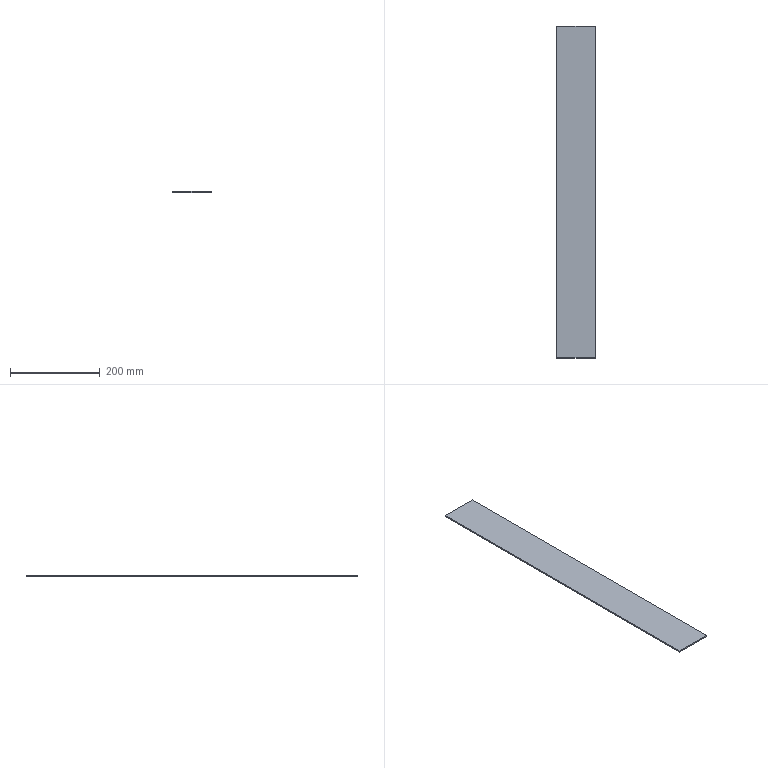Part | STEP file | lll_id4698_x_t | 1 solid | 6 faces | box 85 x 738 x 3 mm | volume 188190 mm3 | plane 6
STEP:
#1=CARTESIAN_POINT('',(174.435,-370.6,0.));
#2=VERTEX_POINT('',#1);
#3=CARTESIAN_POINT('',(89.435,-370.6,0.));
#4=VERTEX_POINT('',#3);
#5=CARTESIAN_POINT('',(197.435,-370.6,0.));
#6=DIRECTION('',(-1.,0.,0.));
#7=VECTOR('',#6,1.);
#8=LINE('',#5,#7);
#9=EDGE_CURVE('',#2,#4,#8,.T.);
#10=ORIENTED_EDGE('',*,*,#9,.F.);
#11=CARTESIAN_POINT('',(174.435,367.4,0.));
#12=VERTEX_POINT('',#11);
#13=CARTESIAN_POINT('',(174.435,0.,0.));
#14=DIRECTION('',(0.,1.,0.));
#15=VECTOR('',#14,1.);
#16=LINE('',#13,#15);
#17=EDGE_CURVE('',#2,#12,#16,.T.);
#18=ORIENTED_EDGE('',*,*,#17,.T.);
#19=CARTESIAN_POINT('',(89.435,367.4,0.));
#20=VERTEX_POINT('',#19);
#21=CARTESIAN_POINT('',(197.435,367.4,0.));
#22=DIRECTION('',(-1.,0.,0.));
#23=VECTOR('',#22,1.);
#24=LINE('',#21,#23);
#25=EDGE_CURVE('',#12,#20,#24,.T.);
#26=ORIENTED_EDGE('',*,*,#25,.T.);
#27=CARTESIAN_POINT('',(89.435,0.,0.));
#28=DIRECTION('',(0.,1.,0.));
#29=VECTOR('',#28,1.);
#30=LINE('',#27,#29);
#31=EDGE_CURVE('',#4,#20,#30,.T.);
#32=ORIENTED_EDGE('',*,*,#31,.F.);
#33=EDGE_LOOP('',(#10,#18,#26,#32));
#34=FACE_OUTER_BOUND('',#33,.T.);
#35=CARTESIAN_POINT('',(197.435,0.,0.));
#36=DIRECTION('',(0.,0.,1.));
#37=DIRECTION('',(0.,-1.,0.));
#38=AXIS2_PLACEMENT_3D('',#35,#36,#37);
#39=PLANE('',#38);
#40=ADVANCED_FACE('',(#34),#39,.T.);
#41=CARTESIAN_POINT('',(89.435,-370.6,-3.));
#42=VERTEX_POINT('',#41);
#43=CARTESIAN_POINT('',(89.435,367.4,-3.));
#44=VERTEX_POINT('',#43);
#45=CARTESIAN_POINT('',(89.435,0.,-3.));
#46=DIRECTION('',(0.,1.,0.));
#47=VECTOR('',#46,1.);
#48=LINE('',#45,#47);
#49=EDGE_CURVE('',#42,#44,#48,.T.);
#50=ORIENTED_EDGE('',*,*,#49,.F.);
#51=CARTESIAN_POINT('',(89.435,-370.6,-80.));
#52=DIRECTION('',(0.,0.,1.));
#53=VECTOR('',#52,1.);
#54=LINE('',#51,#53);
#55=EDGE_CURVE('',#42,#4,#54,.T.);
#56=ORIENTED_EDGE('',*,*,#55,.T.);
#57=ORIENTED_EDGE('',*,*,#31,.T.);
#58=CARTESIAN_POINT('',(89.435,367.4,16.));
#59=DIRECTION('',(0.,0.,1.));
#60=VECTOR('',#59,1.);
#61=LINE('',#58,#60);
#62=EDGE_CURVE('',#44,#20,#61,.T.);
#63=ORIENTED_EDGE('',*,*,#62,.F.);
#64=EDGE_LOOP('',(#50,#56,#57,#63));
#65=FACE_OUTER_BOUND('',#64,.T.);
#66=CARTESIAN_POINT('',(89.435,0.,-80.));
#67=DIRECTION('',(1.,0.,0.));
#68=DIRECTION('',(0.,1.,0.));
#69=AXIS2_PLACEMENT_3D('',#66,#67,#68);
#70=PLANE('',#69);
#71=ADVANCED_FACE('',(#65),#70,.F.);
#72=CARTESIAN_POINT('',(174.435,-370.6,-3.));
#73=VERTEX_POINT('',#72);
#74=CARTESIAN_POINT('',(174.435,-370.6,-80.));
#75=DIRECTION('',(0.,0.,1.));
#76=VECTOR('',#75,1.);
#77=LINE('',#74,#76);
#78=EDGE_CURVE('',#73,#2,#77,.T.);
#79=ORIENTED_EDGE('',*,*,#78,.F.);
#80=CARTESIAN_POINT('',(174.435,367.4,-3.));
#81=VERTEX_POINT('',#80);
#82=CARTESIAN_POINT('',(174.435,0.,-3.));
#83=DIRECTION('',(0.,1.,0.));
#84=VECTOR('',#83,1.);
#85=LINE('',#82,#84);
#86=EDGE_CURVE('',#73,#81,#85,.T.);
#87=ORIENTED_EDGE('',*,*,#86,.T.);
#88=CARTESIAN_POINT('',(174.435,367.4,16.));
#89=DIRECTION('',(0.,0.,1.));
#90=VECTOR('',#89,1.);
#91=LINE('',#88,#90);
#92=EDGE_CURVE('',#81,#12,#91,.T.);
#93=ORIENTED_EDGE('',*,*,#92,.T.);
#94=ORIENTED_EDGE('',*,*,#17,.F.);
#95=EDGE_LOOP('',(#79,#87,#93,#94));
#96=FACE_OUTER_BOUND('',#95,.T.);
#97=CARTESIAN_POINT('',(174.435,0.,-80.));
#98=DIRECTION('',(1.,0.,0.));
#99=DIRECTION('',(0.,1.,0.));
#100=AXIS2_PLACEMENT_3D('',#97,#98,#99);
#101=PLANE('',#100);
#102=ADVANCED_FACE('',(#96),#101,.T.);
#103=CARTESIAN_POINT('',(197.435,-370.6,-3.));
#104=DIRECTION('',(-1.,0.,0.));
#105=VECTOR('',#104,1.);
#106=LINE('',#103,#105);
#107=EDGE_CURVE('',#73,#42,#106,.T.);
#108=ORIENTED_EDGE('',*,*,#107,.F.);
#109=ORIENTED_EDGE('',*,*,#78,.T.);
#110=ORIENTED_EDGE('',*,*,#9,.T.);
#111=ORIENTED_EDGE('',*,*,#55,.F.);
#112=EDGE_LOOP('',(#108,#109,#110,#111));
#113=FACE_OUTER_BOUND('',#112,.T.);
#114=CARTESIAN_POINT('',(197.435,-370.6,16.));
#115=DIRECTION('',(0.,1.,0.));
#116=DIRECTION('',(0.,0.,-1.));
#117=AXIS2_PLACEMENT_3D('',#114,#115,#116);
#118=PLANE('',#117);
#119=ADVANCED_FACE('',(#113),#118,.F.);
#120=CARTESIAN_POINT('',(152.435,367.4,-3.));
#121=DIRECTION('',(-1.,0.,0.));
#122=VECTOR('',#121,1.);
#123=LINE('',#120,#122);
#124=EDGE_CURVE('',#81,#44,#123,.T.);
#125=ORIENTED_EDGE('',*,*,#124,.T.);
#126=ORIENTED_EDGE('',*,*,#62,.T.);
#127=ORIENTED_EDGE('',*,*,#25,.F.);
#128=ORIENTED_EDGE('',*,*,#92,.F.);
#129=EDGE_LOOP('',(#125,#126,#127,#128));
#130=FACE_OUTER_BOUND('',#129,.T.);
#131=CARTESIAN_POINT('',(297.435,367.4,16.));
#132=DIRECTION('',(0.,-1.,0.));
#133=DIRECTION('',(0.,0.,-1.));
#134=AXIS2_PLACEMENT_3D('',#131,#132,#133);
#135=PLANE('',#134);
#136=ADVANCED_FACE('',(#130),#135,.F.);
#137=ORIENTED_EDGE('',*,*,#49,.T.);
#138=ORIENTED_EDGE('',*,*,#124,.F.);
#139=ORIENTED_EDGE('',*,*,#86,.F.);
#140=ORIENTED_EDGE('',*,*,#107,.T.);
#141=EDGE_LOOP('',(#137,#138,#139,#140));
#142=FACE_OUTER_BOUND('',#141,.T.);
#143=CARTESIAN_POINT('',(152.435,0.,-3.));
#144=DIRECTION('',(0.,0.,1.));
#145=DIRECTION('',(1.,0.,0.));
#146=AXIS2_PLACEMENT_3D('',#143,#144,#145);
#147=PLANE('',#146);
#148=ADVANCED_FACE('',(#142),#147,.F.);
#149=CLOSED_SHELL('',(#40,#71,#102,#119,#136,#148));
#150=MANIFOLD_SOLID_BREP('',#149);
#151=(LENGTH_UNIT()NAMED_UNIT(*)SI_UNIT(.MILLI.,.METRE.));
#152=UNCERTAINTY_MEASURE_WITH_UNIT(LENGTH_MEASURE(0.00002),#151,'','');
#153=(NAMED_UNIT(*)PLANE_ANGLE_UNIT()SI_UNIT($,.RADIAN.));
#154=PLANE_ANGLE_MEASURE_WITH_UNIT(PLANE_ANGLE_MEASURE(0.01745),#153);
#155=DIMENSIONAL_EXPONENTS(0.,0.,0.,0.,0.,0.,0.);
#156=(CONVERSION_BASED_UNIT('DEGREE',#154)NAMED_UNIT(#155)PLANE_ANGLE_UNIT());
#157=(NAMED_UNIT(*)SI_UNIT($,.STERADIAN.)SOLID_ANGLE_UNIT());
#158=(GEOMETRIC_REPRESENTATION_CONTEXT(3)GLOBAL_UNCERTAINTY_ASSIGNED_CONTEXT((#152))GLOBAL_UNIT_ASSIGNED_CONTEXT((#151,#156,#157))REPRESENTATION_CONTEXT('',''));
#159=ADVANCED_BREP_SHAPE_REPRESENTATION('',(#150),#158);